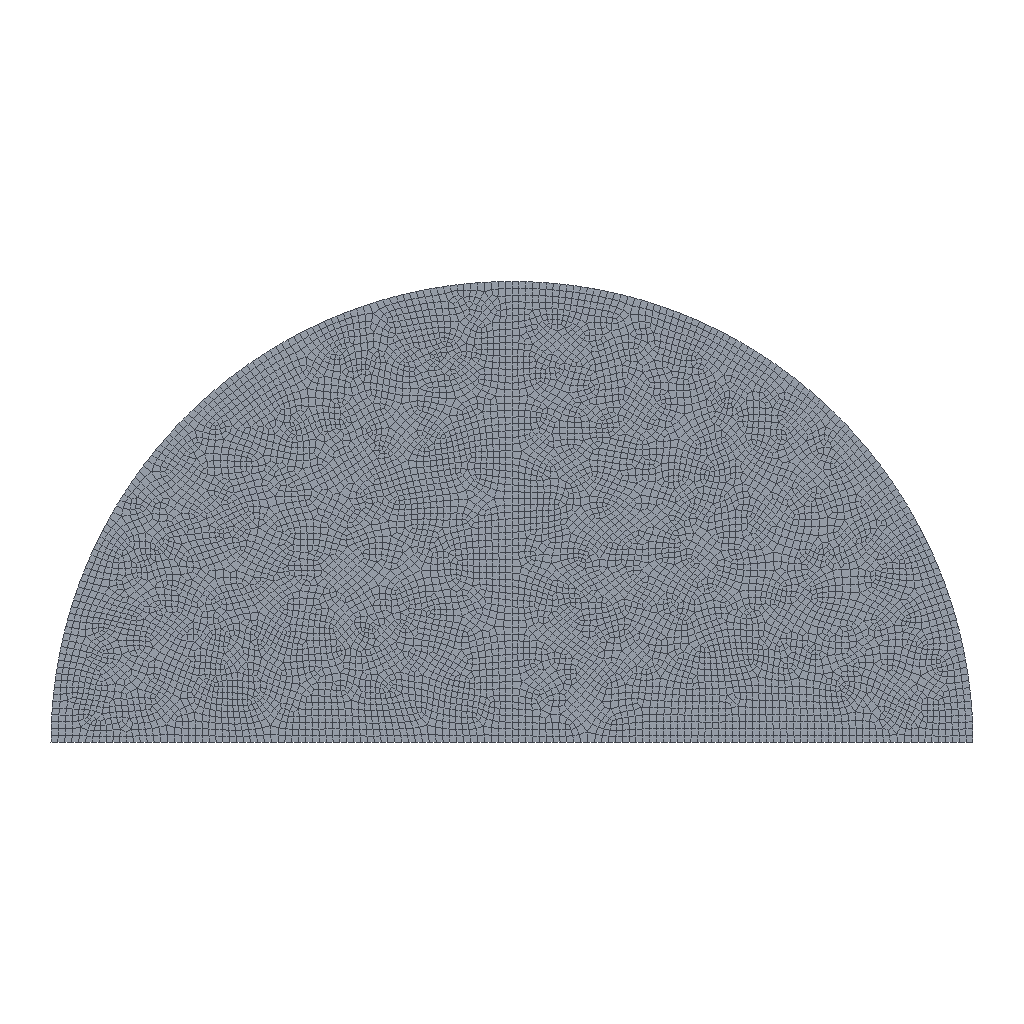Simulation study | abaqus
Set-up summary:
category,name,step,type,value,unit,region
solver,abaqus
solver,version,,,Abaqus/Standard 2020
units,not stated in the deck,,not stated
analysis,deck,,static,static
load_step,Step-1,Step-1,static
load_step,requested,,,1
mesh,nodes,,,8918
mesh,elements,,,8745
element_type,CPS4R,,plane,8745
load,load commands in deck,,count,1
bc,support commands in deck,,count,1
material,MATERIAL-1,,in results
check,setup vs results,,match,"per instance, exact: element labels, types and connectivity; labels of the nodes the elements use; coordinates of those nodes at SINGLE_PRECISION in 1 of 1 instance(s)"
Abaqus input file, long lists of numbers shortened:
*Heading
** Job name: Job-1 Model name: Model-1
** Generated by: Abaqus/CAE 2020
*Preprint, echo=NO, model=NO, history=NO, contact=NO
**
** PARTS
**
*Part, name=Part-1
*Node
      1,           0.,           0.
      2,           0.,          20.
** (8916 more lines like these left out)
*Element, type=CPS4R
   1, 1239, 3875, 1209,  414
   2, 1624, 3921, 1711, 1655
** (8743 more lines like these left out)
*Nset, nset=Set-3, generate
    1,  8918,     1
*Elset, elset=Set-3, generate
    1,  8745,     1
** Section: Section-1
*Solid Section, elset=Set-3, material=Material-1
,
*End Part
**
*Part, name=crack
*End Part
**
**
** ASSEMBLY
**
*Assembly, name=Assembly
**
*Instance, name=Part-1-1, part=Part-1
*End Instance
**
*Instance, name=crack-1, part=crack
1.597, 20.886,           0.
1.597, 20.886,           0., 1.597, 20.886, 1., 10.
*End Instance
**
*Nset, nset=Set-1, instance=Part-1-1
   1,   3,   4, 176, 177, 178, 179, 180, 181, 182, 183, 184, 185, 186, 187, 188
 189, 190, 191, 192, 193, 194, 195, 196, 197, 198, 199, 200, 201, 202, 203, 204
** (7 more lines like these left out)
*Elset, elset=Set-1, instance=Part-1-1
   47,   48,   49,   50,   51,  396,  397,  416,  417,  418,  419,  437,  449,  502,  506,  508
  509,  515,  532,  549,  565,  581,  594,  607,  620,  621,  632,  633,  643,  644,  653,  654
** (7 more lines like these left out)
*Nset, nset=_PickedSet7, internal, instance=Part-1-1, generate
    1,  8918,     1
*Elset, elset=_PickedSet7, internal, instance=Part-1-1, generate
    1,  8745,     1
*Elset, elset=_Surf-1_S3, internal, instance=Part-1-1
   23,   25,   26,   27,   60,  249,  302,  323,  339,  340,  344,  347,  352,  353,  442,  455
  456,  458,  459,  478,  480,  497,  508,  702,  848, 1200, 1231, 1260, 1366, 1436, 1459, 1499
** (2 more lines like these left out)
*Elset, elset=_Surf-1_S1, internal, instance=Part-1-1
   24,   59,   61,  222,  276,  277,  324,  369,  370,  443,  444,  472,  489,  491,  879, 1232
 1258, 1400, 1414, 1415, 1416, 1419, 1425, 1445, 1450, 1468, 1495, 1497, 1498, 1500, 1501, 1502
** (2 more lines like these left out)
*Elset, elset=_Surf-1_S2, internal, instance=Part-1-1
 1469,
*Surface, type=ELEMENT, name=Surf-1
_Surf-1_S3, S3
_Surf-1_S1, S1
_Surf-1_S2, S2
*Enrichment, name=Crack-1, type=PROPAGATION CRACK, elset=_PickedSet7
*End Assembly
*Amplitude, name=Amp-1
             0.,              0.,             0.2,             0.1,             0.4,             0.2,             0.6,             0.9
            0.8,             0.8,              1.,              0.
**
** MATERIALS
**
*Material, name=Material-1
*Damage Initiation, criterion=MAXPS
 0.01,
*Damage Evolution, type=DISPLACEMENT
 1e-10,
*Elastic
226000., 0.3
*Initial Conditions, type=ENRICHMENT
Part-1-1.187, 1,Crack-1, 0.1373, -0.0589
Part-1-1.187, 2,Crack-1, 0.1305, 0.1416
Part-1-1.187, 3,Crack-1, -0.1467, 0.1128
Part-1-1.187, 4,Crack-1, -0.01555, -0.1495
Part-1-1.210, 1,Crack-1, -0.01555
Part-1-1.210, 2,Crack-1, 0.157
Part-1-1.210, 3,Crack-1, 0.3098
Part-1-1.210, 4,Crack-1, 0.1373
Part-1-1.216, 1,Crack-1, -0.1831
Part-1-1.216, 2,Crack-1, -0.02426
Part-1-1.216, 3,Crack-1, 0.157
Part-1-1.216, 4,Crack-1, -0.01555
Part-1-1.167, 1,Crack-1, -0.02426
Part-1-1.167, 2,Crack-1, 0.1662
Part-1-1.167, 3,Crack-1, 0.373
Part-1-1.167, 4,Crack-1, 0.157
Part-1-1.167, 1,Crack-1, -0.1608
Part-1-1.167, 2,Crack-1, 0.1662
Part-1-1.167, 3,Crack-1, -0.02426
Part-1-1.167, 4,Crack-1, -0.2516
Part-1-1.219, 1,Crack-1, 0.1662
Part-1-1.219, 2,Crack-1, -0.1608
Part-1-1.219, 3,Crack-1, -0.1332
Part-1-1.219, 4,Crack-1, 0.09515
Part-1-1.149, 1,Crack-1, -0.03739
Part-1-1.149, 2,Crack-1, 0.09515
Part-1-1.149, 3,Crack-1, -0.1332
Part-1-1.149, 4,Crack-1, -0.3329
Part-1-1.149, 1,Crack-1, 0.2414
Part-1-1.149, 2,Crack-1, 0.3812
Part-1-1.149, 3,Crack-1, 0.09515
Part-1-1.149, 4,Crack-1, -0.03739
Part-1-1.59, 1,Crack-1, 0.09766
Part-1-1.59, 2,Crack-1, 0.2414
Part-1-1.59, 3,Crack-1, -0.03739
Part-1-1.59, 4,Crack-1, -0.1686
Part-1-1.147, 1,Crack-1, -0.3047
Part-1-1.147, 2,Crack-1, -0.05
Part-1-1.147, 3,Crack-1, 0.09766
Part-1-1.147, 4,Crack-1, -0.1686
** ----------------------------------------------------------------
**
** STEP: Step-1
**
*Step, name=Step-1, nlgeom=YES, inc=1000
*Static, stabilize=0.0002, allsdtol=0.05, continue=NO
0.01, 1., 1e-07, 0.1
**
** BOUNDARY CONDITIONS
**
** Name: BC-1 Type: 对称/反对称/完全固定
*Boundary
Set-1, ENCASTRE
**
** LOADS
**
** Name: Load-1   Type: Surface traction
*Dsload, amplitude=Amp-1
Surf-1, TRVEC, 0.01, -0.7071, 0.7071, 0.
**
** CONTROLS
**
*Controls, reset
*Controls, parameters=time incrementation
, , , , , , , 15, , ,
**
** OUTPUT REQUESTS
**
*Restart, write, frequency=0
**
** FIELD OUTPUT: F-Output-1
**
*Output, field
*Node Output
CF, PHILSM, PSILSM, RF, RM, RT, U, V
*Element Output, directions=YES
E, ENRRTXFEM, LE, LOADSXFEM, MISES, MISESMAX, PE, PEEQ, PEMAG, S, SDEG, STATUS, STATUSXFEM
*Contact Output
CDISP, CSTRESS
**
** HISTORY OUTPUT: H-Output-1
**
*Output, history, variable=PRESELECT
*End Step
Results summary:
result,step,,partial,increments=98 time=0.3477/1.0
result,analysis,,,static
result,last_loadstep,,,1
result,primary field,,,U
result,reaction total,,FX,0.03864,model units
result,reaction total,,FY,-0.03829,model units
result,reaction total,,FZ,0.0,model units